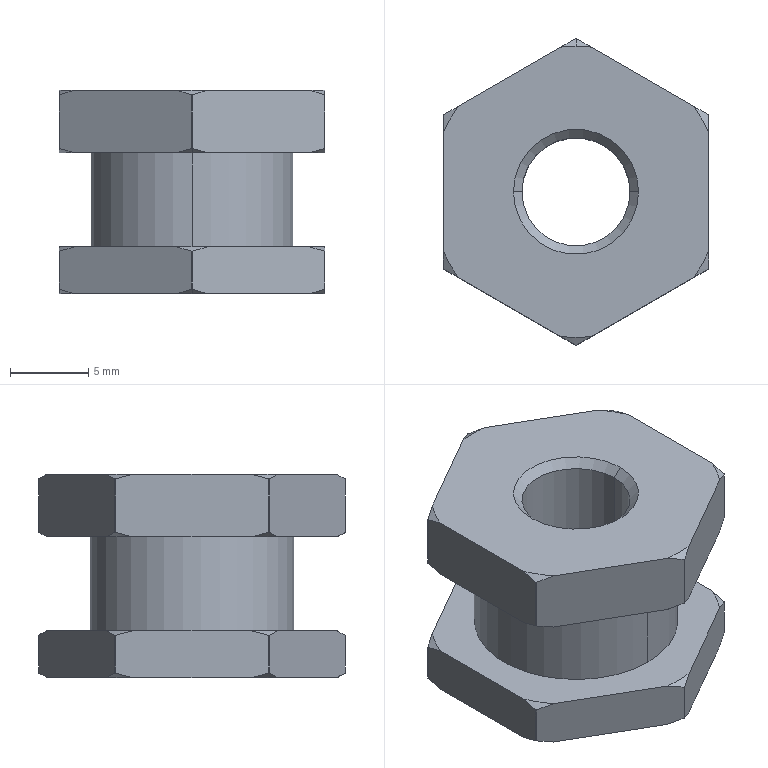Part | SolidWorks | features BaseBody 1 | 1 solid | 66 faces | box 17 x 19.6 x 13 mm | volume 2052 mm3 | cone 32 | cylinder 18 | plane 16 | commonest cylinder face diameters 19.6 x14 6.917 x2 13 x2